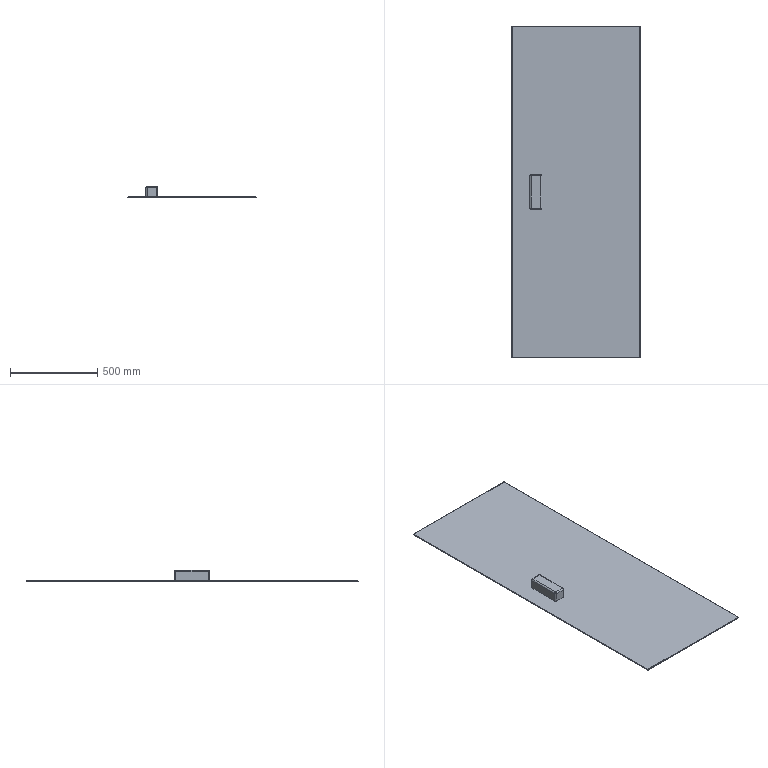Part | SolidWorks | features Fillet 3, EdgeFlange 1, FlatPattern 1, ICE 1, SMBaseFlange 1, SheetMetal 1, Shell 1 | 1 solid | 64 faces | box 735 x 1900 x 64 mm | volume 3179609 mm3 | plane 32 | cylinder 20 | spline 8 | sphere 4 | commonest cylinder face diameters 16 x9 1.473 x4 5.473 x4 2 x3